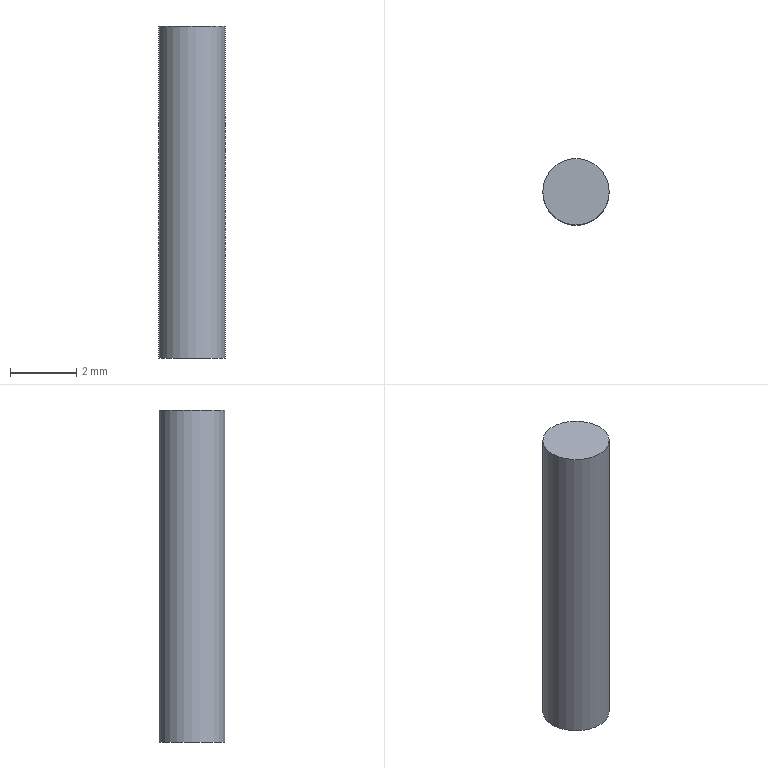Part | NX | features CYLINDER 1, DATUM_CSYS 1 | 1 solid | 3 faces | box 2 x 2 x 10 mm | volume 31.416 mm3 | plane 2 | cylinder 1 | commonest cylinder face diameters 2 x1
STEP:
#1=CARTESIAN_POINT('',(1.,0.,10.));
#2=VERTEX_POINT('',#1);
#3=CARTESIAN_POINT('',(0.,0.,10.));
#4=DIRECTION('',(0.,0.,-1.));
#5=DIRECTION('',(1.,0.,0.));
#6=AXIS2_PLACEMENT_3D('',#3,#4,#5);
#7=CIRCLE('',#6,1.);
#8=EDGE_CURVE('',#2,#2,#7,.T.);
#9=ORIENTED_EDGE('',*,*,#8,.F.);
#10=EDGE_LOOP('',(#9));
#11=FACE_BOUND('',#10,.T.);
#12=CARTESIAN_POINT('',(0.,0.,10.));
#13=DIRECTION('',(0.,0.,1.));
#14=DIRECTION('',(1.,0.,0.));
#15=AXIS2_PLACEMENT_3D('',#12,#13,#14);
#16=PLANE('',#15);
#17=ADVANCED_FACE('',(#11),#16,.T.);
#18=CARTESIAN_POINT('',(1.,0.,0.));
#19=VERTEX_POINT('',#18);
#20=CARTESIAN_POINT('',(0.,0.,0.));
#21=DIRECTION('',(0.,0.,1.));
#22=DIRECTION('',(1.,0.,0.));
#23=AXIS2_PLACEMENT_3D('',#20,#21,#22);
#24=CIRCLE('',#23,1.);
#25=EDGE_CURVE('',#19,#19,#24,.T.);
#26=ORIENTED_EDGE('',*,*,#25,.F.);
#27=EDGE_LOOP('',(#26));
#28=FACE_BOUND('',#27,.T.);
#29=CARTESIAN_POINT('',(0.,0.,0.));
#30=DIRECTION('',(0.,0.,-1.));
#31=DIRECTION('',(-1.,0.,0.));
#32=AXIS2_PLACEMENT_3D('',#29,#30,#31);
#33=PLANE('',#32);
#34=ADVANCED_FACE('',(#28),#33,.T.);
#35=ORIENTED_EDGE('',*,*,#8,.T.);
#36=EDGE_LOOP('',(#35));
#37=FACE_BOUND('',#36,.T.);
#38=ORIENTED_EDGE('',*,*,#25,.T.);
#39=EDGE_LOOP('',(#38));
#40=FACE_BOUND('',#39,.T.);
#41=CARTESIAN_POINT('',(0.,0.,0.));
#42=DIRECTION('',(0.,0.,1.));
#43=DIRECTION('',(1.,0.,0.));
#44=AXIS2_PLACEMENT_3D('',#41,#42,#43);
#45=CYLINDRICAL_SURFACE('',#44,1.);
#46=ADVANCED_FACE('',(#37,#40),#45,.T.);
#47=CLOSED_SHELL('',(#17,#34,#46));
#48=MANIFOLD_SOLID_BREP('',#47);
#49=(LENGTH_UNIT()NAMED_UNIT(*)SI_UNIT(.MILLI.,.METRE.));
#50=UNCERTAINTY_MEASURE_WITH_UNIT(LENGTH_MEASURE(0.00001),#49,'','');
#51=(NAMED_UNIT(*)PLANE_ANGLE_UNIT()SI_UNIT($,.RADIAN.));
#52=(NAMED_UNIT(*)SI_UNIT($,.STERADIAN.)SOLID_ANGLE_UNIT());
#53=(GEOMETRIC_REPRESENTATION_CONTEXT(3)GLOBAL_UNCERTAINTY_ASSIGNED_CONTEXT((#50))GLOBAL_UNIT_ASSIGNED_CONTEXT((#49,#51,#52))REPRESENTATION_CONTEXT('',''));
#54=ADVANCED_BREP_SHAPE_REPRESENTATION('',(#48),#53);